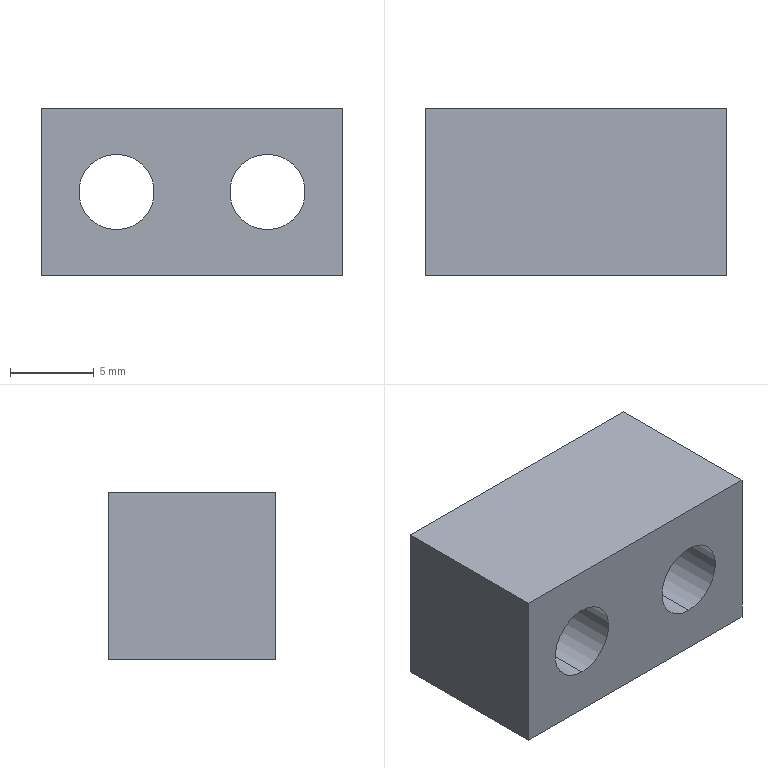Part | STEP file | limit block | 1 solid | 16 faces | box 18 x 10 x 10 mm | volume 1180 mm3 | cylinder 8 | plane 8 | commonest cylinder face diameters 4.5 x4 8 x4
STEP:
#1=CARTESIAN_POINT('',(0.,0.,0.));
#2=DIRECTION('',(0.,0.,1.));
#3=DIRECTION('',(1.,0.,0.));
#4=AXIS2_PLACEMENT_3D('',#1,#2,#3);
#5=CARTESIAN_POINT('',(-4.5,5.6,4.));
#6=VERTEX_POINT('',#5);
#7=CARTESIAN_POINT('',(-4.5,10.,4.));
#8=VERTEX_POINT('',#7);
#9=CARTESIAN_POINT('',(-4.5,10.,4.));
#10=DIRECTION('',(0.,1.,0.));
#11=VECTOR('',#10,1.);
#12=LINE('',#9,#11);
#13=CARTESIAN_POINT('',(-4.5,10.,0.));
#14=DIRECTION('',(0.,1.,0.));
#15=DIRECTION('',(0.,0.,1.));
#16=AXIS2_PLACEMENT_3D('',#13,#14,#15);
#17=CYLINDRICAL_SURFACE('',#16,4.);
#18=CARTESIAN_POINT('',(6.283,0.));
#19=DIRECTION('',(0.,1.));
#20=VECTOR('',#19,1.);
#21=LINE('',#18,#20);
#22=(GEOMETRIC_REPRESENTATION_CONTEXT(2)PARAMETRIC_REPRESENTATION_CONTEXT()REPRESENTATION_CONTEXT('',''));
#23=DEFINITIONAL_REPRESENTATION('',(#21),#22);
#24=PCURVE('',#17,#23);
#25=CARTESIAN_POINT('',(-4.5,10.,0.));
#26=DIRECTION('',(0.,1.,0.));
#27=DIRECTION('',(0.,0.,1.));
#28=AXIS2_PLACEMENT_3D('',#25,#26,#27);
#29=CYLINDRICAL_SURFACE('',#28,4.);
#30=CARTESIAN_POINT('',(0.,0.));
#31=DIRECTION('',(0.,1.));
#32=VECTOR('',#31,1.);
#33=LINE('',#30,#32);
#34=(GEOMETRIC_REPRESENTATION_CONTEXT(2)PARAMETRIC_REPRESENTATION_CONTEXT()REPRESENTATION_CONTEXT('',''));
#35=DEFINITIONAL_REPRESENTATION('',(#33),#34);
#36=PCURVE('',#29,#35);
#37=SURFACE_CURVE('',#12,(#24,#36),.PCURVE_S1.);
#38=EDGE_CURVE('',#6,#8,#37,.T.);
#39=ORIENTED_EDGE('',*,*,#38,.T.);
#40=CARTESIAN_POINT('',(-4.5,10.,-4.));
#41=VERTEX_POINT('',#40);
#42=CARTESIAN_POINT('',(-4.5,10.,0.));
#43=DIRECTION('',(0.,1.,0.));
#44=DIRECTION('',(0.,0.,1.));
#45=AXIS2_PLACEMENT_3D('',#42,#43,#44);
#46=CIRCLE('',#45,4.);
#47=CARTESIAN_POINT('',(0.,0.));
#48=DIRECTION('',(1.,0.));
#49=VECTOR('',#48,1.);
#50=LINE('',#47,#49);
#51=(GEOMETRIC_REPRESENTATION_CONTEXT(2)PARAMETRIC_REPRESENTATION_CONTEXT()REPRESENTATION_CONTEXT('',''));
#52=DEFINITIONAL_REPRESENTATION('',(#50),#51);
#53=PCURVE('',#17,#52);
#54=CARTESIAN_POINT('',(0.,10.,0.));
#55=DIRECTION('',(0.,1.,0.));
#56=DIRECTION('',(0.,0.,1.));
#57=AXIS2_PLACEMENT_3D('',#54,#55,#56);
#58=PLANE('',#57);
#59=CARTESIAN_POINT('',(0.,-4.5));
#60=DIRECTION('',(1.,0.));
#61=AXIS2_PLACEMENT_2D('',#59,#60);
#62=CIRCLE('',#61,4.);
#63=(GEOMETRIC_REPRESENTATION_CONTEXT(2)PARAMETRIC_REPRESENTATION_CONTEXT()REPRESENTATION_CONTEXT('',''));
#64=DEFINITIONAL_REPRESENTATION('',(#62),#63);
#65=PCURVE('',#58,#64);
#66=SURFACE_CURVE('',#46,(#53,#65),.PCURVE_S1.);
#67=EDGE_CURVE('',#41,#8,#66,.T.);
#68=ORIENTED_EDGE('',*,*,#67,.F.);
#69=CARTESIAN_POINT('',(-4.5,5.6,-4.));
#70=VERTEX_POINT('',#69);
#71=CARTESIAN_POINT('',(-4.5,10.,-4.));
#72=DIRECTION('',(0.,1.,0.));
#73=VECTOR('',#72,1.);
#74=LINE('',#71,#73);
#75=CARTESIAN_POINT('',(3.142,0.));
#76=DIRECTION('',(0.,1.));
#77=VECTOR('',#76,1.);
#78=LINE('',#75,#77);
#79=(GEOMETRIC_REPRESENTATION_CONTEXT(2)PARAMETRIC_REPRESENTATION_CONTEXT()REPRESENTATION_CONTEXT('',''));
#80=DEFINITIONAL_REPRESENTATION('',(#78),#79);
#81=PCURVE('',#17,#80);
#82=CARTESIAN_POINT('',(3.142,0.));
#83=DIRECTION('',(0.,1.));
#84=VECTOR('',#83,1.);
#85=LINE('',#82,#84);
#86=(GEOMETRIC_REPRESENTATION_CONTEXT(2)PARAMETRIC_REPRESENTATION_CONTEXT()REPRESENTATION_CONTEXT('',''));
#87=DEFINITIONAL_REPRESENTATION('',(#85),#86);
#88=PCURVE('',#29,#87);
#89=SURFACE_CURVE('',#74,(#81,#88),.PCURVE_S1.);
#90=EDGE_CURVE('',#70,#41,#89,.T.);
#91=ORIENTED_EDGE('',*,*,#90,.F.);
#92=CARTESIAN_POINT('',(-4.5,5.6,0.));
#93=DIRECTION('',(0.,1.,0.));
#94=DIRECTION('',(0.,0.,1.));
#95=AXIS2_PLACEMENT_3D('',#92,#93,#94);
#96=CIRCLE('',#95,4.);
#97=CARTESIAN_POINT('',(0.,-4.4));
#98=DIRECTION('',(1.,0.));
#99=VECTOR('',#98,1.);
#100=LINE('',#97,#99);
#101=(GEOMETRIC_REPRESENTATION_CONTEXT(2)PARAMETRIC_REPRESENTATION_CONTEXT()REPRESENTATION_CONTEXT('',''));
#102=DEFINITIONAL_REPRESENTATION('',(#100),#101);
#103=PCURVE('',#17,#102);
#104=CARTESIAN_POINT('',(-2.25,5.6,0.));
#105=DIRECTION('',(0.,-1.,0.));
#106=DIRECTION('',(0.,0.,-1.));
#107=AXIS2_PLACEMENT_3D('',#104,#105,#106);
#108=PLANE('',#107);
#109=CARTESIAN_POINT('',(-4.,-2.25));
#110=CARTESIAN_POINT('',(-4.,4.678));
#111=CARTESIAN_POINT('',(2.,1.214));
#112=CARTESIAN_POINT('',(8.,-2.25));
#113=CARTESIAN_POINT('',(2.,-5.714));
#114=CARTESIAN_POINT('',(-4.,-9.178));
#115=CARTESIAN_POINT('',(-4.,-2.25));
#116=(BOUNDED_CURVE()B_SPLINE_CURVE(2,(#109,#110,#111,#112,#113,#114,#115),.UNSPECIFIED.,.T.,.F.)B_SPLINE_CURVE_WITH_KNOTS((1,2,2,2,2,1),(-2.094,0.,2.094,4.189,6.283,8.378),.UNSPECIFIED.)CURVE()GEOMETRIC_REPRESENTATION_ITEM()RATIONAL_B_SPLINE_CURVE((1.,0.5,1.,0.5,1.,0.5,1.))REPRESENTATION_ITEM(''));
#117=(GEOMETRIC_REPRESENTATION_CONTEXT(2)PARAMETRIC_REPRESENTATION_CONTEXT()REPRESENTATION_CONTEXT('',''));
#118=DEFINITIONAL_REPRESENTATION('',(#116),#117);
#119=PCURVE('',#108,#118);
#120=SURFACE_CURVE('',#96,(#103,#119),.PCURVE_S1.);
#121=EDGE_CURVE('',#70,#6,#120,.T.);
#122=ORIENTED_EDGE('',*,*,#121,.T.);
#123=EDGE_LOOP('',(#39,#68,#91,#122));
#124=FACE_BOUND('',#123,.F.);
#125=ADVANCED_FACE('',(#124),#17,.F.);
#126=CARTESIAN_POINT('',(-4.5,0.,2.25));
#127=VERTEX_POINT('',#126);
#128=CARTESIAN_POINT('',(-4.5,5.6,2.25));
#129=VERTEX_POINT('',#128);
#130=CARTESIAN_POINT('',(-4.5,10.,2.25));
#131=DIRECTION('',(0.,1.,0.));
#132=VECTOR('',#131,1.);
#133=LINE('',#130,#132);
#134=CARTESIAN_POINT('',(-4.5,10.,0.));
#135=DIRECTION('',(0.,1.,0.));
#136=DIRECTION('',(0.,0.,1.));
#137=AXIS2_PLACEMENT_3D('',#134,#135,#136);
#138=CYLINDRICAL_SURFACE('',#137,2.25);
#139=CARTESIAN_POINT('',(6.283,0.));
#140=DIRECTION('',(0.,1.));
#141=VECTOR('',#140,1.);
#142=LINE('',#139,#141);
#143=(GEOMETRIC_REPRESENTATION_CONTEXT(2)PARAMETRIC_REPRESENTATION_CONTEXT()REPRESENTATION_CONTEXT('',''));
#144=DEFINITIONAL_REPRESENTATION('',(#142),#143);
#145=PCURVE('',#138,#144);
#146=CARTESIAN_POINT('',(-4.5,10.,0.));
#147=DIRECTION('',(0.,1.,0.));
#148=DIRECTION('',(0.,0.,1.));
#149=AXIS2_PLACEMENT_3D('',#146,#147,#148);
#150=CYLINDRICAL_SURFACE('',#149,2.25);
#151=CARTESIAN_POINT('',(0.,0.));
#152=DIRECTION('',(0.,1.));
#153=VECTOR('',#152,1.);
#154=LINE('',#151,#153);
#155=(GEOMETRIC_REPRESENTATION_CONTEXT(2)PARAMETRIC_REPRESENTATION_CONTEXT()REPRESENTATION_CONTEXT('',''));
#156=DEFINITIONAL_REPRESENTATION('',(#154),#155);
#157=PCURVE('',#150,#156);
#158=SURFACE_CURVE('',#133,(#145,#157),.PCURVE_S1.);
#159=EDGE_CURVE('',#127,#129,#158,.T.);
#160=ORIENTED_EDGE('',*,*,#159,.T.);
#161=CARTESIAN_POINT('',(-4.5,5.6,-2.25));
#162=VERTEX_POINT('',#161);
#163=CARTESIAN_POINT('',(-4.5,5.6,0.));
#164=DIRECTION('',(0.,1.,0.));
#165=DIRECTION('',(0.,0.,1.));
#166=AXIS2_PLACEMENT_3D('',#163,#164,#165);
#167=CIRCLE('',#166,2.25);
#168=CARTESIAN_POINT('',(0.,-4.4));
#169=DIRECTION('',(1.,0.));
#170=VECTOR('',#169,1.);
#171=LINE('',#168,#170);
#172=(GEOMETRIC_REPRESENTATION_CONTEXT(2)PARAMETRIC_REPRESENTATION_CONTEXT()REPRESENTATION_CONTEXT('',''));
#173=DEFINITIONAL_REPRESENTATION('',(#171),#172);
#174=PCURVE('',#138,#173);
#175=CARTESIAN_POINT('',(-2.25,-2.25));
#176=CARTESIAN_POINT('',(-2.25,1.647));
#177=CARTESIAN_POINT('',(1.125,-0.3014));
#178=CARTESIAN_POINT('',(4.5,-2.25));
#179=CARTESIAN_POINT('',(1.125,-4.199));
#180=CARTESIAN_POINT('',(-2.25,-6.147));
#181=CARTESIAN_POINT('',(-2.25,-2.25));
#182=(BOUNDED_CURVE()B_SPLINE_CURVE(2,(#175,#176,#177,#178,#179,#180,#181),.UNSPECIFIED.,.T.,.F.)B_SPLINE_CURVE_WITH_KNOTS((1,2,2,2,2,1),(-2.094,0.,2.094,4.189,6.283,8.378),.UNSPECIFIED.)CURVE()GEOMETRIC_REPRESENTATION_ITEM()RATIONAL_B_SPLINE_CURVE((1.,0.5,1.,0.5,1.,0.5,1.))REPRESENTATION_ITEM(''));
#183=(GEOMETRIC_REPRESENTATION_CONTEXT(2)PARAMETRIC_REPRESENTATION_CONTEXT()REPRESENTATION_CONTEXT('',''));
#184=DEFINITIONAL_REPRESENTATION('',(#182),#183);
#185=PCURVE('',#108,#184);
#186=SURFACE_CURVE('',#167,(#174,#185),.PCURVE_S1.);
#187=EDGE_CURVE('',#162,#129,#186,.T.);
#188=ORIENTED_EDGE('',*,*,#187,.F.);
#189=CARTESIAN_POINT('',(-4.5,0.,-2.25));
#190=VERTEX_POINT('',#189);
#191=CARTESIAN_POINT('',(-4.5,10.,-2.25));
#192=DIRECTION('',(0.,1.,0.));
#193=VECTOR('',#192,1.);
#194=LINE('',#191,#193);
#195=CARTESIAN_POINT('',(3.142,0.));
#196=DIRECTION('',(0.,1.));
#197=VECTOR('',#196,1.);
#198=LINE('',#195,#197);
#199=(GEOMETRIC_REPRESENTATION_CONTEXT(2)PARAMETRIC_REPRESENTATION_CONTEXT()REPRESENTATION_CONTEXT('',''));
#200=DEFINITIONAL_REPRESENTATION('',(#198),#199);
#201=PCURVE('',#138,#200);
#202=CARTESIAN_POINT('',(3.142,0.));
#203=DIRECTION('',(0.,1.));
#204=VECTOR('',#203,1.);
#205=LINE('',#202,#204);
#206=(GEOMETRIC_REPRESENTATION_CONTEXT(2)PARAMETRIC_REPRESENTATION_CONTEXT()REPRESENTATION_CONTEXT('',''));
#207=DEFINITIONAL_REPRESENTATION('',(#205),#206);
#208=PCURVE('',#150,#207);
#209=SURFACE_CURVE('',#194,(#201,#208),.PCURVE_S1.);
#210=EDGE_CURVE('',#190,#162,#209,.T.);
#211=ORIENTED_EDGE('',*,*,#210,.F.);
#212=CARTESIAN_POINT('',(-4.5,0.,0.));
#213=DIRECTION('',(0.,1.,0.));
#214=DIRECTION('',(0.,0.,1.));
#215=AXIS2_PLACEMENT_3D('',#212,#213,#214);
#216=CIRCLE('',#215,2.25);
#217=CARTESIAN_POINT('',(0.,-10.));
#218=DIRECTION('',(1.,0.));
#219=VECTOR('',#218,1.);
#220=LINE('',#217,#219);
#221=(GEOMETRIC_REPRESENTATION_CONTEXT(2)PARAMETRIC_REPRESENTATION_CONTEXT()REPRESENTATION_CONTEXT('',''));
#222=DEFINITIONAL_REPRESENTATION('',(#220),#221);
#223=PCURVE('',#138,#222);
#224=CARTESIAN_POINT('',(0.,0.,0.));
#225=DIRECTION('',(0.,1.,0.));
#226=DIRECTION('',(0.,0.,1.));
#227=AXIS2_PLACEMENT_3D('',#224,#225,#226);
#228=PLANE('',#227);
#229=CARTESIAN_POINT('',(0.,-4.5));
#230=DIRECTION('',(1.,0.));
#231=AXIS2_PLACEMENT_2D('',#229,#230);
#232=CIRCLE('',#231,2.25);
#233=(GEOMETRIC_REPRESENTATION_CONTEXT(2)PARAMETRIC_REPRESENTATION_CONTEXT()REPRESENTATION_CONTEXT('',''));
#234=DEFINITIONAL_REPRESENTATION('',(#232),#233);
#235=PCURVE('',#228,#234);
#236=SURFACE_CURVE('',#216,(#223,#235),.PCURVE_S1.);
#237=EDGE_CURVE('',#190,#127,#236,.T.);
#238=ORIENTED_EDGE('',*,*,#237,.T.);
#239=EDGE_LOOP('',(#160,#188,#211,#238));
#240=FACE_BOUND('',#239,.F.);
#241=ADVANCED_FACE('',(#240),#138,.F.);
#242=CARTESIAN_POINT('',(4.5,5.6,4.));
#243=VERTEX_POINT('',#242);
#244=CARTESIAN_POINT('',(4.5,10.,4.));
#245=VERTEX_POINT('',#244);
#246=CARTESIAN_POINT('',(4.5,10.,4.));
#247=DIRECTION('',(0.,1.,0.));
#248=VECTOR('',#247,1.);
#249=LINE('',#246,#248);
#250=CARTESIAN_POINT('',(4.5,10.,0.));
#251=DIRECTION('',(0.,1.,0.));
#252=DIRECTION('',(0.,0.,1.));
#253=AXIS2_PLACEMENT_3D('',#250,#251,#252);
#254=CYLINDRICAL_SURFACE('',#253,4.);
#255=CARTESIAN_POINT('',(6.283,0.));
#256=DIRECTION('',(0.,1.));
#257=VECTOR('',#256,1.);
#258=LINE('',#255,#257);
#259=(GEOMETRIC_REPRESENTATION_CONTEXT(2)PARAMETRIC_REPRESENTATION_CONTEXT()REPRESENTATION_CONTEXT('',''));
#260=DEFINITIONAL_REPRESENTATION('',(#258),#259);
#261=PCURVE('',#254,#260);
#262=CARTESIAN_POINT('',(4.5,10.,0.));
#263=DIRECTION('',(0.,1.,0.));
#264=DIRECTION('',(0.,0.,1.));
#265=AXIS2_PLACEMENT_3D('',#262,#263,#264);
#266=CYLINDRICAL_SURFACE('',#265,4.);
#267=CARTESIAN_POINT('',(0.,0.));
#268=DIRECTION('',(0.,1.));
#269=VECTOR('',#268,1.);
#270=LINE('',#267,#269);
#271=(GEOMETRIC_REPRESENTATION_CONTEXT(2)PARAMETRIC_REPRESENTATION_CONTEXT()REPRESENTATION_CONTEXT('',''));
#272=DEFINITIONAL_REPRESENTATION('',(#270),#271);
#273=PCURVE('',#266,#272);
#274=SURFACE_CURVE('',#249,(#261,#273),.PCURVE_S1.);
#275=EDGE_CURVE('',#243,#245,#274,.T.);
#276=ORIENTED_EDGE('',*,*,#275,.T.);
#277=CARTESIAN_POINT('',(4.5,10.,-4.));
#278=VERTEX_POINT('',#277);
#279=CARTESIAN_POINT('',(4.5,10.,0.));
#280=DIRECTION('',(0.,1.,0.));
#281=DIRECTION('',(0.,0.,1.));
#282=AXIS2_PLACEMENT_3D('',#279,#280,#281);
#283=CIRCLE('',#282,4.);
#284=CARTESIAN_POINT('',(0.,0.));
#285=DIRECTION('',(1.,0.));
#286=VECTOR('',#285,1.);
#287=LINE('',#284,#286);
#288=(GEOMETRIC_REPRESENTATION_CONTEXT(2)PARAMETRIC_REPRESENTATION_CONTEXT()REPRESENTATION_CONTEXT('',''));
#289=DEFINITIONAL_REPRESENTATION('',(#287),#288);
#290=PCURVE('',#254,#289);
#291=CARTESIAN_POINT('',(0.,4.5));
#292=DIRECTION('',(1.,0.));
#293=AXIS2_PLACEMENT_2D('',#291,#292);
#294=CIRCLE('',#293,4.);
#295=(GEOMETRIC_REPRESENTATION_CONTEXT(2)PARAMETRIC_REPRESENTATION_CONTEXT()REPRESENTATION_CONTEXT('',''));
#296=DEFINITIONAL_REPRESENTATION('',(#294),#295);
#297=PCURVE('',#58,#296);
#298=SURFACE_CURVE('',#283,(#290,#297),.PCURVE_S1.);
#299=EDGE_CURVE('',#278,#245,#298,.T.);
#300=ORIENTED_EDGE('',*,*,#299,.F.);
#301=CARTESIAN_POINT('',(4.5,5.6,-4.));
#302=VERTEX_POINT('',#301);
#303=CARTESIAN_POINT('',(4.5,10.,-4.));
#304=DIRECTION('',(0.,1.,0.));
#305=VECTOR('',#304,1.);
#306=LINE('',#303,#305);
#307=CARTESIAN_POINT('',(3.142,0.));
#308=DIRECTION('',(0.,1.));
#309=VECTOR('',#308,1.);
#310=LINE('',#307,#309);
#311=(GEOMETRIC_REPRESENTATION_CONTEXT(2)PARAMETRIC_REPRESENTATION_CONTEXT()REPRESENTATION_CONTEXT('',''));
#312=DEFINITIONAL_REPRESENTATION('',(#310),#311);
#313=PCURVE('',#254,#312);
#314=CARTESIAN_POINT('',(3.142,0.));
#315=DIRECTION('',(0.,1.));
#316=VECTOR('',#315,1.);
#317=LINE('',#314,#316);
#318=(GEOMETRIC_REPRESENTATION_CONTEXT(2)PARAMETRIC_REPRESENTATION_CONTEXT()REPRESENTATION_CONTEXT('',''));
#319=DEFINITIONAL_REPRESENTATION('',(#317),#318);
#320=PCURVE('',#266,#319);
#321=SURFACE_CURVE('',#306,(#313,#320),.PCURVE_S1.);
#322=EDGE_CURVE('',#302,#278,#321,.T.);
#323=ORIENTED_EDGE('',*,*,#322,.F.);
#324=CARTESIAN_POINT('',(4.5,5.6,0.));
#325=DIRECTION('',(0.,1.,0.));
#326=DIRECTION('',(0.,0.,1.));
#327=AXIS2_PLACEMENT_3D('',#324,#325,#326);
#328=CIRCLE('',#327,4.);
#329=CARTESIAN_POINT('',(0.,-4.4));
#330=DIRECTION('',(1.,0.));
#331=VECTOR('',#330,1.);
#332=LINE('',#329,#331);
#333=(GEOMETRIC_REPRESENTATION_CONTEXT(2)PARAMETRIC_REPRESENTATION_CONTEXT()REPRESENTATION_CONTEXT('',''));
#334=DEFINITIONAL_REPRESENTATION('',(#332),#333);
#335=PCURVE('',#254,#334);
#336=CARTESIAN_POINT('',(6.75,5.6,0.));
#337=DIRECTION('',(0.,-1.,0.));
#338=DIRECTION('',(0.,0.,-1.));
#339=AXIS2_PLACEMENT_3D('',#336,#337,#338);
#340=PLANE('',#339);
#341=CARTESIAN_POINT('',(-4.,-2.25));
#342=CARTESIAN_POINT('',(-4.,4.678));
#343=CARTESIAN_POINT('',(2.,1.214));
#344=CARTESIAN_POINT('',(8.,-2.25));
#345=CARTESIAN_POINT('',(2.,-5.714));
#346=CARTESIAN_POINT('',(-4.,-9.178));
#347=CARTESIAN_POINT('',(-4.,-2.25));
#348=(BOUNDED_CURVE()B_SPLINE_CURVE(2,(#341,#342,#343,#344,#345,#346,#347),.UNSPECIFIED.,.T.,.F.)B_SPLINE_CURVE_WITH_KNOTS((1,2,2,2,2,1),(-2.094,0.,2.094,4.189,6.283,8.378),.UNSPECIFIED.)CURVE()GEOMETRIC_REPRESENTATION_ITEM()RATIONAL_B_SPLINE_CURVE((1.,0.5,1.,0.5,1.,0.5,1.))REPRESENTATION_ITEM(''));
#349=(GEOMETRIC_REPRESENTATION_CONTEXT(2)PARAMETRIC_REPRESENTATION_CONTEXT()REPRESENTATION_CONTEXT('',''));
#350=DEFINITIONAL_REPRESENTATION('',(#348),#349);
#351=PCURVE('',#340,#350);
#352=SURFACE_CURVE('',#328,(#335,#351),.PCURVE_S1.);
#353=EDGE_CURVE('',#302,#243,#352,.T.);
#354=ORIENTED_EDGE('',*,*,#353,.T.);
#355=EDGE_LOOP('',(#276,#300,#323,#354));
#356=FACE_BOUND('',#355,.F.);
#357=ADVANCED_FACE('',(#356),#254,.F.);
#358=CARTESIAN_POINT('',(4.5,0.,2.25));
#359=VERTEX_POINT('',#358);
#360=CARTESIAN_POINT('',(4.5,5.6,2.25));
#361=VERTEX_POINT('',#360);
#362=CARTESIAN_POINT('',(4.5,10.,2.25));
#363=DIRECTION('',(0.,1.,0.));
#364=VECTOR('',#363,1.);
#365=LINE('',#362,#364);
#366=CARTESIAN_POINT('',(4.5,10.,0.));
#367=DIRECTION('',(0.,1.,0.));
#368=DIRECTION('',(0.,0.,1.));
#369=AXIS2_PLACEMENT_3D('',#366,#367,#368);
#370=CYLINDRICAL_SURFACE('',#369,2.25);
#371=CARTESIAN_POINT('',(6.283,0.));
#372=DIRECTION('',(0.,1.));
#373=VECTOR('',#372,1.);
#374=LINE('',#371,#373);
#375=(GEOMETRIC_REPRESENTATION_CONTEXT(2)PARAMETRIC_REPRESENTATION_CONTEXT()REPRESENTATION_CONTEXT('',''));
#376=DEFINITIONAL_REPRESENTATION('',(#374),#375);
#377=PCURVE('',#370,#376);
#378=CARTESIAN_POINT('',(4.5,10.,0.));
#379=DIRECTION('',(0.,1.,0.));
#380=DIRECTION('',(0.,0.,1.));
#381=AXIS2_PLACEMENT_3D('',#378,#379,#380);
#382=CYLINDRICAL_SURFACE('',#381,2.25);
#383=CARTESIAN_POINT('',(0.,0.));
#384=DIRECTION('',(0.,1.));
#385=VECTOR('',#384,1.);
#386=LINE('',#383,#385);
#387=(GEOMETRIC_REPRESENTATION_CONTEXT(2)PARAMETRIC_REPRESENTATION_CONTEXT()REPRESENTATION_CONTEXT('',''));
#388=DEFINITIONAL_REPRESENTATION('',(#386),#387);
#389=PCURVE('',#382,#388);
#390=SURFACE_CURVE('',#365,(#377,#389),.PCURVE_S1.);
#391=EDGE_CURVE('',#359,#361,#390,.T.);
#392=ORIENTED_EDGE('',*,*,#391,.T.);
#393=CARTESIAN_POINT('',(4.5,5.6,-2.25));
#394=VERTEX_POINT('',#393);
#395=CARTESIAN_POINT('',(4.5,5.6,0.));
#396=DIRECTION('',(0.,1.,0.));
#397=DIRECTION('',(0.,0.,1.));
#398=AXIS2_PLACEMENT_3D('',#395,#396,#397);
#399=CIRCLE('',#398,2.25);
#400=CARTESIAN_POINT('',(0.,-4.4));
#401=DIRECTION('',(1.,0.));
#402=VECTOR('',#401,1.);
#403=LINE('',#400,#402);
#404=(GEOMETRIC_REPRESENTATION_CONTEXT(2)PARAMETRIC_REPRESENTATION_CONTEXT()REPRESENTATION_CONTEXT('',''));
#405=DEFINITIONAL_REPRESENTATION('',(#403),#404);
#406=PCURVE('',#370,#405);
#407=CARTESIAN_POINT('',(-2.25,-2.25));
#408=CARTESIAN_POINT('',(-2.25,1.647));
#409=CARTESIAN_POINT('',(1.125,-0.3014));
#410=CARTESIAN_POINT('',(4.5,-2.25));
#411=CARTESIAN_POINT('',(1.125,-4.199));
#412=CARTESIAN_POINT('',(-2.25,-6.147));
#413=CARTESIAN_POINT('',(-2.25,-2.25));
#414=(BOUNDED_CURVE()B_SPLINE_CURVE(2,(#407,#408,#409,#410,#411,#412,#413),.UNSPECIFIED.,.T.,.F.)B_SPLINE_CURVE_WITH_KNOTS((1,2,2,2,2,1),(-2.094,0.,2.094,4.189,6.283,8.378),.UNSPECIFIED.)CURVE()GEOMETRIC_REPRESENTATION_ITEM()RATIONAL_B_SPLINE_CURVE((1.,0.5,1.,0.5,1.,0.5,1.))REPRESENTATION_ITEM(''));
#415=(GEOMETRIC_REPRESENTATION_CONTEXT(2)PARAMETRIC_REPRESENTATION_CONTEXT()REPRESENTATION_CONTEXT('',''));
#416=DEFINITIONAL_REPRESENTATION('',(#414),#415);
#417=PCURVE('',#340,#416);
#418=SURFACE_CURVE('',#399,(#406,#417),.PCURVE_S1.);
#419=EDGE_CURVE('',#394,#361,#418,.T.);
#420=ORIENTED_EDGE('',*,*,#419,.F.);
#421=CARTESIAN_POINT('',(4.5,0.,-2.25));
#422=VERTEX_POINT('',#421);
#423=CARTESIAN_POINT('',(4.5,10.,-2.25));
#424=DIRECTION('',(0.,1.,0.));
#425=VECTOR('',#424,1.);
#426=LINE('',#423,#425);
#427=CARTESIAN_POINT('',(3.142,0.));
#428=DIRECTION('',(0.,1.));
#429=VECTOR('',#428,1.);
#430=LINE('',#427,#429);
#431=(GEOMETRIC_REPRESENTATION_CONTEXT(2)PARAMETRIC_REPRESENTATION_CONTEXT()REPRESENTATION_CONTEXT('',''));
#432=DEFINITIONAL_REPRESENTATION('',(#430),#431);
#433=PCURVE('',#370,#432);
#434=CARTESIAN_POINT('',(3.142,0.));
#435=DIRECTION('',(0.,1.));
#436=VECTOR('',#435,1.);
#437=LINE('',#434,#436);
#438=(GEOMETRIC_REPRESENTATION_CONTEXT(2)PARAMETRIC_REPRESENTATION_CONTEXT()REPRESENTATION_CONTEXT('',''));
#439=DEFINITIONAL_REPRESENTATION('',(#437),#438);
#440=PCURVE('',#382,#439);
#441=SURFACE_CURVE('',#426,(#433,#440),.PCURVE_S1.);
#442=EDGE_CURVE('',#422,#394,#441,.T.);
#443=ORIENTED_EDGE('',*,*,#442,.F.);
#444=CARTESIAN_POINT('',(4.5,0.,0.));
#445=DIRECTION('',(0.,1.,0.));
#446=DIRECTION('',(0.,0.,1.));
#447=AXIS2_PLACEMENT_3D('',#444,#445,#446);
#448=CIRCLE('',#447,2.25);
#449=CARTESIAN_POINT('',(0.,-10.));
#450=DIRECTION('',(1.,0.));
#451=VECTOR('',#450,1.);
#452=LINE('',#449,#451);
#453=(GEOMETRIC_REPRESENTATION_CONTEXT(2)PARAMETRIC_REPRESENTATION_CONTEXT()REPRESENTATION_CONTEXT('',''));
#454=DEFINITIONAL_REPRESENTATION('',(#452),#453);
#455=PCURVE('',#370,#454);
#456=CARTESIAN_POINT('',(0.,4.5));
#457=DIRECTION('',(1.,0.));
#458=AXIS2_PLACEMENT_2D('',#456,#457);
#459=CIRCLE('',#458,2.25);
#460=(GEOMETRIC_REPRESENTATION_CONTEXT(2)PARAMETRIC_REPRESENTATION_CONTEXT()REPRESENTATION_CONTEXT('',''));
#461=DEFINITIONAL_REPRESENTATION('',(#459),#460);
#462=PCURVE('',#228,#461);
#463=SURFACE_CURVE('',#448,(#455,#462),.PCURVE_S1.);
#464=EDGE_CURVE('',#422,#359,#463,.T.);
#465=ORIENTED_EDGE('',*,*,#464,.T.);
#466=EDGE_LOOP('',(#392,#420,#443,#465));
#467=FACE_BOUND('',#466,.F.);
#468=ADVANCED_FACE('',(#467),#370,.F.);
#469=CARTESIAN_POINT('',(9.,0.,5.));
#470=VERTEX_POINT('',#469);
#471=CARTESIAN_POINT('',(9.,0.,-5.));
#472=VERTEX_POINT('',#471);
#473=CARTESIAN_POINT('',(9.,0.,-5.));
#474=DIRECTION('',(0.,0.,-1.));
#475=VECTOR('',#474,1.);
#476=LINE('',#473,#475);
#477=CARTESIAN_POINT('',(9.,10.,-5.));
#478=DIRECTION('',(-1.,0.,0.));
#479=DIRECTION('',(0.,0.,1.));
#480=AXIS2_PLACEMENT_3D('',#477,#478,#479);
#481=PLANE('',#480);
#482=CARTESIAN_POINT('',(0.,-10.));
#483=DIRECTION('',(-1.,0.));
#484=VECTOR('',#483,1.);
#485=LINE('',#482,#484);
#486=(GEOMETRIC_REPRESENTATION_CONTEXT(2)PARAMETRIC_REPRESENTATION_CONTEXT()REPRESENTATION_CONTEXT('',''));
#487=DEFINITIONAL_REPRESENTATION('',(#485),#486);
#488=PCURVE('',#481,#487);
#489=CARTESIAN_POINT('',(-5.,9.));
#490=DIRECTION('',(-1.,0.));
#491=VECTOR('',#490,1.);
#492=LINE('',#489,#491);
#493=(GEOMETRIC_REPRESENTATION_CONTEXT(2)PARAMETRIC_REPRESENTATION_CONTEXT()REPRESENTATION_CONTEXT('',''));
#494=DEFINITIONAL_REPRESENTATION('',(#492),#493);
#495=PCURVE('',#228,#494);
#496=SURFACE_CURVE('',#476,(#488,#495),.PCURVE_S1.);
#497=EDGE_CURVE('',#470,#472,#496,.T.);
#498=ORIENTED_EDGE('',*,*,#497,.T.);
#499=CARTESIAN_POINT('',(9.,10.,-5.));
#500=VERTEX_POINT('',#499);
#501=CARTESIAN_POINT('',(9.,10.,-5.));
#502=DIRECTION('',(0.,-1.,0.));
#503=VECTOR('',#502,1.);
#504=LINE('',#501,#503);
#505=CARTESIAN_POINT('',(0.,0.));
#506=DIRECTION('',(0.,-1.));
#507=VECTOR('',#506,1.);
#508=LINE('',#505,#507);
#509=(GEOMETRIC_REPRESENTATION_CONTEXT(2)PARAMETRIC_REPRESENTATION_CONTEXT()REPRESENTATION_CONTEXT('',''));
#510=DEFINITIONAL_REPRESENTATION('',(#508),#509);
#511=PCURVE('',#481,#510);
#512=CARTESIAN_POINT('',(-9.,10.,-5.));
#513=DIRECTION('',(0.,0.,1.));
#514=DIRECTION('',(1.,0.,0.));
#515=AXIS2_PLACEMENT_3D('',#512,#513,#514);
#516=PLANE('',#515);
#517=CARTESIAN_POINT('',(18.,0.));
#518=DIRECTION('',(0.,-1.));
#519=VECTOR('',#518,1.);
#520=LINE('',#517,#519);
#521=(GEOMETRIC_REPRESENTATION_CONTEXT(2)PARAMETRIC_REPRESENTATION_CONTEXT()REPRESENTATION_CONTEXT('',''));
#522=DEFINITIONAL_REPRESENTATION('',(#520),#521);
#523=PCURVE('',#516,#522);
#524=SURFACE_CURVE('',#504,(#511,#523),.PCURVE_S1.);
#525=EDGE_CURVE('',#500,#472,#524,.T.);
#526=ORIENTED_EDGE('',*,*,#525,.F.);
#527=CARTESIAN_POINT('',(9.,10.,5.));
#528=VERTEX_POINT('',#527);
#529=CARTESIAN_POINT('',(9.,10.,-5.));
#530=DIRECTION('',(0.,0.,-1.));
#531=VECTOR('',#530,1.);
#532=LINE('',#529,#531);
#533=CARTESIAN_POINT('',(0.,0.));
#534=DIRECTION('',(-1.,0.));
#535=VECTOR('',#534,1.);
#536=LINE('',#533,#535);
#537=(GEOMETRIC_REPRESENTATION_CONTEXT(2)PARAMETRIC_REPRESENTATION_CONTEXT()REPRESENTATION_CONTEXT('',''));
#538=DEFINITIONAL_REPRESENTATION('',(#536),#537);
#539=PCURVE('',#481,#538);
#540=CARTESIAN_POINT('',(-5.,9.));
#541=DIRECTION('',(-1.,0.));
#542=VECTOR('',#541,1.);
#543=LINE('',#540,#542);
#544=(GEOMETRIC_REPRESENTATION_CONTEXT(2)PARAMETRIC_REPRESENTATION_CONTEXT()REPRESENTATION_CONTEXT('',''));
#545=DEFINITIONAL_REPRESENTATION('',(#543),#544);
#546=PCURVE('',#58,#545);
#547=SURFACE_CURVE('',#532,(#539,#546),.PCURVE_S1.);
#548=EDGE_CURVE('',#528,#500,#547,.T.);
#549=ORIENTED_EDGE('',*,*,#548,.F.);
#550=CARTESIAN_POINT('',(9.,10.,5.));
#551=DIRECTION('',(0.,-1.,0.));
#552=VECTOR('',#551,1.);
#553=LINE('',#550,#552);
#554=CARTESIAN_POINT('',(10.,0.));
#555=DIRECTION('',(0.,-1.));
#556=VECTOR('',#555,1.);
#557=LINE('',#554,#556);
#558=(GEOMETRIC_REPRESENTATION_CONTEXT(2)PARAMETRIC_REPRESENTATION_CONTEXT()REPRESENTATION_CONTEXT('',''));
#559=DEFINITIONAL_REPRESENTATION('',(#557),#558);
#560=PCURVE('',#481,#559);
#561=CARTESIAN_POINT('',(-9.,10.,5.));
#562=DIRECTION('',(0.,0.,-1.));
#563=DIRECTION('',(-1.,0.,0.));
#564=AXIS2_PLACEMENT_3D('',#561,#562,#563);
#565=PLANE('',#564);
#566=CARTESIAN_POINT('',(-18.,0.));
#567=DIRECTION('',(0.,-1.));
#568=VECTOR('',#567,1.);
#569=LINE('',#566,#568);
#570=(GEOMETRIC_REPRESENTATION_CONTEXT(2)PARAMETRIC_REPRESENTATION_CONTEXT()REPRESENTATION_CONTEXT('',''));
#571=DEFINITIONAL_REPRESENTATION('',(#569),#570);
#572=PCURVE('',#565,#571);
#573=SURFACE_CURVE('',#553,(#560,#572),.PCURVE_S1.);
#574=EDGE_CURVE('',#528,#470,#573,.T.);
#575=ORIENTED_EDGE('',*,*,#574,.T.);
#576=EDGE_LOOP('',(#498,#526,#549,#575));
#577=FACE_BOUND('',#576,.T.);
#578=ADVANCED_FACE('',(#577),#481,.F.);
#579=CARTESIAN_POINT('',(-9.,0.,-5.));
#580=VERTEX_POINT('',#579);
#581=CARTESIAN_POINT('',(-9.,0.,-5.));
#582=DIRECTION('',(-1.,0.,0.));
#583=VECTOR('',#582,1.);
#584=LINE('',#581,#583);
#585=CARTESIAN_POINT('',(0.,-10.));
#586=DIRECTION('',(-1.,0.));
#587=VECTOR('',#586,1.);
#588=LINE('',#585,#587);
#589=(GEOMETRIC_REPRESENTATION_CONTEXT(2)PARAMETRIC_REPRESENTATION_CONTEXT()REPRESENTATION_CONTEXT('',''));
#590=DEFINITIONAL_REPRESENTATION('',(#588),#589);
#591=PCURVE('',#516,#590);
#592=CARTESIAN_POINT('',(-5.,-9.));
#593=DIRECTION('',(0.,-1.));
#594=VECTOR('',#593,1.);
#595=LINE('',#592,#594);
#596=(GEOMETRIC_REPRESENTATION_CONTEXT(2)PARAMETRIC_REPRESENTATION_CONTEXT()REPRESENTATION_CONTEXT('',''));
#597=DEFINITIONAL_REPRESENTATION('',(#595),#596);
#598=PCURVE('',#228,#597);
#599=SURFACE_CURVE('',#584,(#591,#598),.PCURVE_S1.);
#600=EDGE_CURVE('',#472,#580,#599,.T.);
#601=ORIENTED_EDGE('',*,*,#600,.T.);
#602=CARTESIAN_POINT('',(-9.,10.,-5.));
#603=VERTEX_POINT('',#602);
#604=CARTESIAN_POINT('',(-9.,10.,-5.));
#605=DIRECTION('',(0.,-1.,0.));
#606=VECTOR('',#605,1.);
#607=LINE('',#604,#606);
#608=CARTESIAN_POINT('',(0.,0.));
#609=DIRECTION('',(0.,-1.));
#610=VECTOR('',#609,1.);
#611=LINE('',#608,#610);
#612=(GEOMETRIC_REPRESENTATION_CONTEXT(2)PARAMETRIC_REPRESENTATION_CONTEXT()REPRESENTATION_CONTEXT('',''));
#613=DEFINITIONAL_REPRESENTATION('',(#611),#612);
#614=PCURVE('',#516,#613);
#615=CARTESIAN_POINT('',(-9.,10.,-5.));
#616=DIRECTION('',(1.,0.,0.));
#617=DIRECTION('',(0.,0.,-1.));
#618=AXIS2_PLACEMENT_3D('',#615,#616,#617);
#619=PLANE('',#618);
#620=CARTESIAN_POINT('',(0.,0.));
#621=DIRECTION('',(0.,-1.));
#622=VECTOR('',#621,1.);
#623=LINE('',#620,#622);
#624=(GEOMETRIC_REPRESENTATION_CONTEXT(2)PARAMETRIC_REPRESENTATION_CONTEXT()REPRESENTATION_CONTEXT('',''));
#625=DEFINITIONAL_REPRESENTATION('',(#623),#624);
#626=PCURVE('',#619,#625);
#627=SURFACE_CURVE('',#607,(#614,#626),.PCURVE_S1.);
#628=EDGE_CURVE('',#603,#580,#627,.T.);
#629=ORIENTED_EDGE('',*,*,#628,.F.);
#630=CARTESIAN_POINT('',(-9.,10.,-5.));
#631=DIRECTION('',(-1.,0.,0.));
#632=VECTOR('',#631,1.);
#633=LINE('',#630,#632);
#634=CARTESIAN_POINT('',(0.,0.));
#635=DIRECTION('',(-1.,0.));
#636=VECTOR('',#635,1.);
#637=LINE('',#634,#636);
#638=(GEOMETRIC_REPRESENTATION_CONTEXT(2)PARAMETRIC_REPRESENTATION_CONTEXT()REPRESENTATION_CONTEXT('',''));
#639=DEFINITIONAL_REPRESENTATION('',(#637),#638);
#640=PCURVE('',#516,#639);
#641=CARTESIAN_POINT('',(-5.,-9.));
#642=DIRECTION('',(0.,-1.));
#643=VECTOR('',#642,1.);
#644=LINE('',#641,#643);
#645=(GEOMETRIC_REPRESENTATION_CONTEXT(2)PARAMETRIC_REPRESENTATION_CONTEXT()REPRESENTATION_CONTEXT('',''));
#646=DEFINITIONAL_REPRESENTATION('',(#644),#645);
#647=PCURVE('',#58,#646);
#648=SURFACE_CURVE('',#633,(#640,#647),.PCURVE_S1.);
#649=EDGE_CURVE('',#500,#603,#648,.T.);
#650=ORIENTED_EDGE('',*,*,#649,.F.);
#651=ORIENTED_EDGE('',*,*,#525,.T.);
#652=EDGE_LOOP('',(#601,#629,#650,#651));
#653=FACE_BOUND('',#652,.T.);
#654=ADVANCED_FACE('',(#653),#516,.F.);
#655=CARTESIAN_POINT('',(-9.,0.,5.));
#656=VERTEX_POINT('',#655);
#657=CARTESIAN_POINT('',(-9.,0.,-5.));
#658=DIRECTION('',(0.,0.,1.));
#659=VECTOR('',#658,1.);
#660=LINE('',#657,#659);
#661=CARTESIAN_POINT('',(0.,-10.));
#662=DIRECTION('',(-1.,0.));
#663=VECTOR('',#662,1.);
#664=LINE('',#661,#663);
#665=(GEOMETRIC_REPRESENTATION_CONTEXT(2)PARAMETRIC_REPRESENTATION_CONTEXT()REPRESENTATION_CONTEXT('',''));
#666=DEFINITIONAL_REPRESENTATION('',(#664),#665);
#667=PCURVE('',#619,#666);
#668=CARTESIAN_POINT('',(-5.,-9.));
#669=DIRECTION('',(1.,0.));
#670=VECTOR('',#669,1.);
#671=LINE('',#668,#670);
#672=(GEOMETRIC_REPRESENTATION_CONTEXT(2)PARAMETRIC_REPRESENTATION_CONTEXT()REPRESENTATION_CONTEXT('',''));
#673=DEFINITIONAL_REPRESENTATION('',(#671),#672);
#674=PCURVE('',#228,#673);
#675=SURFACE_CURVE('',#660,(#667,#674),.PCURVE_S1.);
#676=EDGE_CURVE('',#580,#656,#675,.T.);
#677=ORIENTED_EDGE('',*,*,#676,.T.);
#678=CARTESIAN_POINT('',(-9.,10.,5.));
#679=VERTEX_POINT('',#678);
#680=CARTESIAN_POINT('',(-9.,10.,5.));
#681=DIRECTION('',(0.,-1.,0.));
#682=VECTOR('',#681,1.);
#683=LINE('',#680,#682);
#684=CARTESIAN_POINT('',(-10.,0.));
#685=DIRECTION('',(0.,-1.));
#686=VECTOR('',#685,1.);
#687=LINE('',#684,#686);
#688=(GEOMETRIC_REPRESENTATION_CONTEXT(2)PARAMETRIC_REPRESENTATION_CONTEXT()REPRESENTATION_CONTEXT('',''));
#689=DEFINITIONAL_REPRESENTATION('',(#687),#688);
#690=PCURVE('',#619,#689);
#691=CARTESIAN_POINT('',(0.,0.));
#692=DIRECTION('',(0.,-1.));
#693=VECTOR('',#692,1.);
#694=LINE('',#691,#693);
#695=(GEOMETRIC_REPRESENTATION_CONTEXT(2)PARAMETRIC_REPRESENTATION_CONTEXT()REPRESENTATION_CONTEXT('',''));
#696=DEFINITIONAL_REPRESENTATION('',(#694),#695);
#697=PCURVE('',#565,#696);
#698=SURFACE_CURVE('',#683,(#690,#697),.PCURVE_S1.);
#699=EDGE_CURVE('',#679,#656,#698,.T.);
#700=ORIENTED_EDGE('',*,*,#699,.F.);
#701=CARTESIAN_POINT('',(-9.,10.,-5.));
#702=DIRECTION('',(0.,0.,1.));
#703=VECTOR('',#702,1.);
#704=LINE('',#701,#703);
#705=CARTESIAN_POINT('',(0.,0.));
#706=DIRECTION('',(-1.,0.));
#707=VECTOR('',#706,1.);
#708=LINE('',#705,#707);
#709=(GEOMETRIC_REPRESENTATION_CONTEXT(2)PARAMETRIC_REPRESENTATION_CONTEXT()REPRESENTATION_CONTEXT('',''));
#710=DEFINITIONAL_REPRESENTATION('',(#708),#709);
#711=PCURVE('',#619,#710);
#712=CARTESIAN_POINT('',(-5.,-9.));
#713=DIRECTION('',(1.,0.));
#714=VECTOR('',#713,1.);
#715=LINE('',#712,#714);
#716=(GEOMETRIC_REPRESENTATION_CONTEXT(2)PARAMETRIC_REPRESENTATION_CONTEXT()REPRESENTATION_CONTEXT('',''));
#717=DEFINITIONAL_REPRESENTATION('',(#715),#716);
#718=PCURVE('',#58,#717);
#719=SURFACE_CURVE('',#704,(#711,#718),.PCURVE_S1.);
#720=EDGE_CURVE('',#603,#679,#719,.T.);
#721=ORIENTED_EDGE('',*,*,#720,.F.);
#722=ORIENTED_EDGE('',*,*,#628,.T.);
#723=EDGE_LOOP('',(#677,#700,#721,#722));
#724=FACE_BOUND('',#723,.T.);
#725=ADVANCED_FACE('',(#724),#619,.F.);
#726=CARTESIAN_POINT('',(-9.,0.,5.));
#727=DIRECTION('',(1.,0.,0.));
#728=VECTOR('',#727,1.);
#729=LINE('',#726,#728);
#730=CARTESIAN_POINT('',(0.,-10.));
#731=DIRECTION('',(-1.,0.));
#732=VECTOR('',#731,1.);
#733=LINE('',#730,#732);
#734=(GEOMETRIC_REPRESENTATION_CONTEXT(2)PARAMETRIC_REPRESENTATION_CONTEXT()REPRESENTATION_CONTEXT('',''));
#735=DEFINITIONAL_REPRESENTATION('',(#733),#734);
#736=PCURVE('',#565,#735);
#737=CARTESIAN_POINT('',(5.,-9.));
#738=DIRECTION('',(0.,1.));
#739=VECTOR('',#738,1.);
#740=LINE('',#737,#739);
#741=(GEOMETRIC_REPRESENTATION_CONTEXT(2)PARAMETRIC_REPRESENTATION_CONTEXT()REPRESENTATION_CONTEXT('',''));
#742=DEFINITIONAL_REPRESENTATION('',(#740),#741);
#743=PCURVE('',#228,#742);
#744=SURFACE_CURVE('',#729,(#736,#743),.PCURVE_S1.);
#745=EDGE_CURVE('',#656,#470,#744,.T.);
#746=ORIENTED_EDGE('',*,*,#745,.T.);
#747=ORIENTED_EDGE('',*,*,#574,.F.);
#748=CARTESIAN_POINT('',(-9.,10.,5.));
#749=DIRECTION('',(1.,0.,0.));
#750=VECTOR('',#749,1.);
#751=LINE('',#748,#750);
#752=CARTESIAN_POINT('',(0.,0.));
#753=DIRECTION('',(-1.,0.));
#754=VECTOR('',#753,1.);
#755=LINE('',#752,#754);
#756=(GEOMETRIC_REPRESENTATION_CONTEXT(2)PARAMETRIC_REPRESENTATION_CONTEXT()REPRESENTATION_CONTEXT('',''));
#757=DEFINITIONAL_REPRESENTATION('',(#755),#756);
#758=PCURVE('',#565,#757);
#759=CARTESIAN_POINT('',(5.,-9.));
#760=DIRECTION('',(0.,1.));
#761=VECTOR('',#760,1.);
#762=LINE('',#759,#761);
#763=(GEOMETRIC_REPRESENTATION_CONTEXT(2)PARAMETRIC_REPRESENTATION_CONTEXT()REPRESENTATION_CONTEXT('',''));
#764=DEFINITIONAL_REPRESENTATION('',(#762),#763);
#765=PCURVE('',#58,#764);
#766=SURFACE_CURVE('',#751,(#758,#765),.PCURVE_S1.);
#767=EDGE_CURVE('',#679,#528,#766,.T.);
#768=ORIENTED_EDGE('',*,*,#767,.F.);
#769=ORIENTED_EDGE('',*,*,#699,.T.);
#770=EDGE_LOOP('',(#746,#747,#768,#769));
#771=FACE_BOUND('',#770,.T.);
#772=ADVANCED_FACE('',(#771),#565,.F.);
#773=CARTESIAN_POINT('',(-4.5,10.,0.));
#774=DIRECTION('',(0.,1.,0.));
#775=DIRECTION('',(0.,0.,1.));
#776=AXIS2_PLACEMENT_3D('',#773,#774,#775);
#777=CIRCLE('',#776,4.);
#778=CARTESIAN_POINT('',(0.,-4.5));
#779=DIRECTION('',(1.,0.));
#780=AXIS2_PLACEMENT_2D('',#778,#779);
#781=CIRCLE('',#780,4.);
#782=(GEOMETRIC_REPRESENTATION_CONTEXT(2)PARAMETRIC_REPRESENTATION_CONTEXT()REPRESENTATION_CONTEXT('',''));
#783=DEFINITIONAL_REPRESENTATION('',(#781),#782);
#784=PCURVE('',#58,#783);
#785=CARTESIAN_POINT('',(0.,0.));
#786=DIRECTION('',(1.,0.));
#787=VECTOR('',#786,1.);
#788=LINE('',#785,#787);
#789=(GEOMETRIC_REPRESENTATION_CONTEXT(2)PARAMETRIC_REPRESENTATION_CONTEXT()REPRESENTATION_CONTEXT('',''));
#790=DEFINITIONAL_REPRESENTATION('',(#788),#789);
#791=PCURVE('',#29,#790);
#792=SURFACE_CURVE('',#777,(#784,#791),.PCURVE_S1.);
#793=EDGE_CURVE('',#8,#41,#792,.T.);
#794=ORIENTED_EDGE('',*,*,#793,.F.);
#795=ORIENTED_EDGE('',*,*,#67,.F.);
#796=EDGE_LOOP('',(#794,#795));
#797=FACE_BOUND('',#796,.T.);
#798=CARTESIAN_POINT('',(4.5,10.,0.));
#799=DIRECTION('',(0.,1.,0.));
#800=DIRECTION('',(0.,0.,1.));
#801=AXIS2_PLACEMENT_3D('',#798,#799,#800);
#802=CIRCLE('',#801,4.);
#803=CARTESIAN_POINT('',(0.,4.5));
#804=DIRECTION('',(1.,0.));
#805=AXIS2_PLACEMENT_2D('',#803,#804);
#806=CIRCLE('',#805,4.);
#807=(GEOMETRIC_REPRESENTATION_CONTEXT(2)PARAMETRIC_REPRESENTATION_CONTEXT()REPRESENTATION_CONTEXT('',''));
#808=DEFINITIONAL_REPRESENTATION('',(#806),#807);
#809=PCURVE('',#58,#808);
#810=CARTESIAN_POINT('',(0.,0.));
#811=DIRECTION('',(1.,0.));
#812=VECTOR('',#811,1.);
#813=LINE('',#810,#812);
#814=(GEOMETRIC_REPRESENTATION_CONTEXT(2)PARAMETRIC_REPRESENTATION_CONTEXT()REPRESENTATION_CONTEXT('',''));
#815=DEFINITIONAL_REPRESENTATION('',(#813),#814);
#816=PCURVE('',#266,#815);
#817=SURFACE_CURVE('',#802,(#809,#816),.PCURVE_S1.);
#818=EDGE_CURVE('',#245,#278,#817,.T.);
#819=ORIENTED_EDGE('',*,*,#818,.F.);
#820=ORIENTED_EDGE('',*,*,#299,.F.);
#821=EDGE_LOOP('',(#819,#820));
#822=FACE_BOUND('',#821,.T.);
#823=ORIENTED_EDGE('',*,*,#548,.T.);
#824=ORIENTED_EDGE('',*,*,#649,.T.);
#825=ORIENTED_EDGE('',*,*,#720,.T.);
#826=ORIENTED_EDGE('',*,*,#767,.T.);
#827=EDGE_LOOP('',(#823,#824,#825,#826));
#828=FACE_BOUND('',#827,.T.);
#829=ADVANCED_FACE('',(#797,#822,#828),#58,.T.);
#830=CARTESIAN_POINT('',(-4.5,0.,0.));
#831=DIRECTION('',(0.,1.,0.));
#832=DIRECTION('',(0.,0.,1.));
#833=AXIS2_PLACEMENT_3D('',#830,#831,#832);
#834=CIRCLE('',#833,2.25);
#835=CARTESIAN_POINT('',(0.,-4.5));
#836=DIRECTION('',(1.,0.));
#837=AXIS2_PLACEMENT_2D('',#835,#836);
#838=CIRCLE('',#837,2.25);
#839=(GEOMETRIC_REPRESENTATION_CONTEXT(2)PARAMETRIC_REPRESENTATION_CONTEXT()REPRESENTATION_CONTEXT('',''));
#840=DEFINITIONAL_REPRESENTATION('',(#838),#839);
#841=PCURVE('',#228,#840);
#842=CARTESIAN_POINT('',(0.,-10.));
#843=DIRECTION('',(1.,0.));
#844=VECTOR('',#843,1.);
#845=LINE('',#842,#844);
#846=(GEOMETRIC_REPRESENTATION_CONTEXT(2)PARAMETRIC_REPRESENTATION_CONTEXT()REPRESENTATION_CONTEXT('',''));
#847=DEFINITIONAL_REPRESENTATION('',(#845),#846);
#848=PCURVE('',#150,#847);
#849=SURFACE_CURVE('',#834,(#841,#848),.PCURVE_S1.);
#850=EDGE_CURVE('',#127,#190,#849,.T.);
#851=ORIENTED_EDGE('',*,*,#850,.T.);
#852=ORIENTED_EDGE('',*,*,#237,.T.);
#853=EDGE_LOOP('',(#851,#852));
#854=FACE_BOUND('',#853,.T.);
#855=CARTESIAN_POINT('',(4.5,0.,0.));
#856=DIRECTION('',(0.,1.,0.));
#857=DIRECTION('',(0.,0.,1.));
#858=AXIS2_PLACEMENT_3D('',#855,#856,#857);
#859=CIRCLE('',#858,2.25);
#860=CARTESIAN_POINT('',(0.,4.5));
#861=DIRECTION('',(1.,0.));
#862=AXIS2_PLACEMENT_2D('',#860,#861);
#863=CIRCLE('',#862,2.25);
#864=(GEOMETRIC_REPRESENTATION_CONTEXT(2)PARAMETRIC_REPRESENTATION_CONTEXT()REPRESENTATION_CONTEXT('',''));
#865=DEFINITIONAL_REPRESENTATION('',(#863),#864);
#866=PCURVE('',#228,#865);
#867=CARTESIAN_POINT('',(0.,-10.));
#868=DIRECTION('',(1.,0.));
#869=VECTOR('',#868,1.);
#870=LINE('',#867,#869);
#871=(GEOMETRIC_REPRESENTATION_CONTEXT(2)PARAMETRIC_REPRESENTATION_CONTEXT()REPRESENTATION_CONTEXT('',''));
#872=DEFINITIONAL_REPRESENTATION('',(#870),#871);
#873=PCURVE('',#382,#872);
#874=SURFACE_CURVE('',#859,(#866,#873),.PCURVE_S1.);
#875=EDGE_CURVE('',#359,#422,#874,.T.);
#876=ORIENTED_EDGE('',*,*,#875,.T.);
#877=ORIENTED_EDGE('',*,*,#464,.T.);
#878=EDGE_LOOP('',(#876,#877));
#879=FACE_BOUND('',#878,.T.);
#880=ORIENTED_EDGE('',*,*,#497,.F.);
#881=ORIENTED_EDGE('',*,*,#745,.F.);
#882=ORIENTED_EDGE('',*,*,#676,.F.);
#883=ORIENTED_EDGE('',*,*,#600,.F.);
#884=EDGE_LOOP('',(#880,#881,#882,#883));
#885=FACE_BOUND('',#884,.T.);
#886=ADVANCED_FACE('',(#854,#879,#885),#228,.F.);
#887=CARTESIAN_POINT('',(4.5,5.6,0.));
#888=DIRECTION('',(0.,1.,0.));
#889=DIRECTION('',(0.,0.,1.));
#890=AXIS2_PLACEMENT_3D('',#887,#888,#889);
#891=CIRCLE('',#890,2.25);
#892=CARTESIAN_POINT('',(0.,-4.4));
#893=DIRECTION('',(1.,0.));
#894=VECTOR('',#893,1.);
#895=LINE('',#892,#894);
#896=(GEOMETRIC_REPRESENTATION_CONTEXT(2)PARAMETRIC_REPRESENTATION_CONTEXT()REPRESENTATION_CONTEXT('',''));
#897=DEFINITIONAL_REPRESENTATION('',(#895),#896);
#898=PCURVE('',#382,#897);
#899=CARTESIAN_POINT('',(-2.25,-2.25));
#900=CARTESIAN_POINT('',(-2.25,1.647));
#901=CARTESIAN_POINT('',(1.125,-0.3014));
#902=CARTESIAN_POINT('',(4.5,-2.25));
#903=CARTESIAN_POINT('',(1.125,-4.199));
#904=CARTESIAN_POINT('',(-2.25,-6.147));
#905=CARTESIAN_POINT('',(-2.25,-2.25));
#906=(BOUNDED_CURVE()B_SPLINE_CURVE(2,(#899,#900,#901,#902,#903,#904,#905),.UNSPECIFIED.,.T.,.F.)B_SPLINE_CURVE_WITH_KNOTS((1,2,2,2,2,1),(-2.094,0.,2.094,4.189,6.283,8.378),.UNSPECIFIED.)CURVE()GEOMETRIC_REPRESENTATION_ITEM()RATIONAL_B_SPLINE_CURVE((1.,0.5,1.,0.5,1.,0.5,1.))REPRESENTATION_ITEM(''));
#907=(GEOMETRIC_REPRESENTATION_CONTEXT(2)PARAMETRIC_REPRESENTATION_CONTEXT()REPRESENTATION_CONTEXT('',''));
#908=DEFINITIONAL_REPRESENTATION('',(#906),#907);
#909=PCURVE('',#340,#908);
#910=SURFACE_CURVE('',#891,(#898,#909),.PCURVE_S1.);
#911=EDGE_CURVE('',#361,#394,#910,.T.);
#912=ORIENTED_EDGE('',*,*,#911,.F.);
#913=ORIENTED_EDGE('',*,*,#391,.F.);
#914=ORIENTED_EDGE('',*,*,#875,.T.);
#915=ORIENTED_EDGE('',*,*,#442,.T.);
#916=EDGE_LOOP('',(#912,#913,#914,#915));
#917=FACE_BOUND('',#916,.F.);
#918=ADVANCED_FACE('',(#917),#382,.F.);
#919=ORIENTED_EDGE('',*,*,#911,.F.);
#920=ORIENTED_EDGE('',*,*,#419,.F.);
#921=EDGE_LOOP('',(#919,#920));
#922=FACE_BOUND('',#921,.T.);
#923=CARTESIAN_POINT('',(4.5,5.6,0.));
#924=DIRECTION('',(0.,1.,0.));
#925=DIRECTION('',(0.,0.,1.));
#926=AXIS2_PLACEMENT_3D('',#923,#924,#925);
#927=CIRCLE('',#926,4.);
#928=CARTESIAN_POINT('',(-4.,-2.25));
#929=CARTESIAN_POINT('',(-4.,4.678));
#930=CARTESIAN_POINT('',(2.,1.214));
#931=CARTESIAN_POINT('',(8.,-2.25));
#932=CARTESIAN_POINT('',(2.,-5.714));
#933=CARTESIAN_POINT('',(-4.,-9.178));
#934=CARTESIAN_POINT('',(-4.,-2.25));
#935=(BOUNDED_CURVE()B_SPLINE_CURVE(2,(#928,#929,#930,#931,#932,#933,#934),.UNSPECIFIED.,.T.,.F.)B_SPLINE_CURVE_WITH_KNOTS((1,2,2,2,2,1),(-2.094,0.,2.094,4.189,6.283,8.378),.UNSPECIFIED.)CURVE()GEOMETRIC_REPRESENTATION_ITEM()RATIONAL_B_SPLINE_CURVE((1.,0.5,1.,0.5,1.,0.5,1.))REPRESENTATION_ITEM(''));
#936=(GEOMETRIC_REPRESENTATION_CONTEXT(2)PARAMETRIC_REPRESENTATION_CONTEXT()REPRESENTATION_CONTEXT('',''));
#937=DEFINITIONAL_REPRESENTATION('',(#935),#936);
#938=PCURVE('',#340,#937);
#939=CARTESIAN_POINT('',(0.,-4.4));
#940=DIRECTION('',(1.,0.));
#941=VECTOR('',#940,1.);
#942=LINE('',#939,#941);
#943=(GEOMETRIC_REPRESENTATION_CONTEXT(2)PARAMETRIC_REPRESENTATION_CONTEXT()REPRESENTATION_CONTEXT('',''));
#944=DEFINITIONAL_REPRESENTATION('',(#942),#943);
#945=PCURVE('',#266,#944);
#946=SURFACE_CURVE('',#927,(#938,#945),.PCURVE_S1.);
#947=EDGE_CURVE('',#243,#302,#946,.T.);
#948=ORIENTED_EDGE('',*,*,#947,.T.);
#949=ORIENTED_EDGE('',*,*,#353,.T.);
#950=EDGE_LOOP('',(#948,#949));
#951=FACE_BOUND('',#950,.T.);
#952=ADVANCED_FACE('',(#922,#951),#340,.F.);
#953=ORIENTED_EDGE('',*,*,#818,.F.);
#954=ORIENTED_EDGE('',*,*,#275,.F.);
#955=ORIENTED_EDGE('',*,*,#947,.T.);
#956=ORIENTED_EDGE('',*,*,#322,.T.);
#957=EDGE_LOOP('',(#953,#954,#955,#956));
#958=FACE_BOUND('',#957,.F.);
#959=ADVANCED_FACE('',(#958),#266,.F.);
#960=CARTESIAN_POINT('',(-4.5,5.6,0.));
#961=DIRECTION('',(0.,1.,0.));
#962=DIRECTION('',(0.,0.,1.));
#963=AXIS2_PLACEMENT_3D('',#960,#961,#962);
#964=CIRCLE('',#963,2.25);
#965=CARTESIAN_POINT('',(0.,-4.4));
#966=DIRECTION('',(1.,0.));
#967=VECTOR('',#966,1.);
#968=LINE('',#965,#967);
#969=(GEOMETRIC_REPRESENTATION_CONTEXT(2)PARAMETRIC_REPRESENTATION_CONTEXT()REPRESENTATION_CONTEXT('',''));
#970=DEFINITIONAL_REPRESENTATION('',(#968),#969);
#971=PCURVE('',#150,#970);
#972=CARTESIAN_POINT('',(-2.25,-2.25));
#973=CARTESIAN_POINT('',(-2.25,1.647));
#974=CARTESIAN_POINT('',(1.125,-0.3014));
#975=CARTESIAN_POINT('',(4.5,-2.25));
#976=CARTESIAN_POINT('',(1.125,-4.199));
#977=CARTESIAN_POINT('',(-2.25,-6.147));
#978=CARTESIAN_POINT('',(-2.25,-2.25));
#979=(BOUNDED_CURVE()B_SPLINE_CURVE(2,(#972,#973,#974,#975,#976,#977,#978),.UNSPECIFIED.,.T.,.F.)B_SPLINE_CURVE_WITH_KNOTS((1,2,2,2,2,1),(-2.094,0.,2.094,4.189,6.283,8.378),.UNSPECIFIED.)CURVE()GEOMETRIC_REPRESENTATION_ITEM()RATIONAL_B_SPLINE_CURVE((1.,0.5,1.,0.5,1.,0.5,1.))REPRESENTATION_ITEM(''));
#980=(GEOMETRIC_REPRESENTATION_CONTEXT(2)PARAMETRIC_REPRESENTATION_CONTEXT()REPRESENTATION_CONTEXT('',''));
#981=DEFINITIONAL_REPRESENTATION('',(#979),#980);
#982=PCURVE('',#108,#981);
#983=SURFACE_CURVE('',#964,(#971,#982),.PCURVE_S1.);
#984=EDGE_CURVE('',#129,#162,#983,.T.);
#985=ORIENTED_EDGE('',*,*,#984,.F.);
#986=ORIENTED_EDGE('',*,*,#159,.F.);
#987=ORIENTED_EDGE('',*,*,#850,.T.);
#988=ORIENTED_EDGE('',*,*,#210,.T.);
#989=EDGE_LOOP('',(#985,#986,#987,#988));
#990=FACE_BOUND('',#989,.F.);
#991=ADVANCED_FACE('',(#990),#150,.F.);
#992=ORIENTED_EDGE('',*,*,#984,.F.);
#993=ORIENTED_EDGE('',*,*,#187,.F.);
#994=EDGE_LOOP('',(#992,#993));
#995=FACE_BOUND('',#994,.T.);
#996=CARTESIAN_POINT('',(-4.5,5.6,0.));
#997=DIRECTION('',(0.,1.,0.));
#998=DIRECTION('',(0.,0.,1.));
#999=AXIS2_PLACEMENT_3D('',#996,#997,#998);
#1000=CIRCLE('',#999,4.);
#1001=CARTESIAN_POINT('',(-4.,-2.25));
#1002=CARTESIAN_POINT('',(-4.,4.678));
#1003=CARTESIAN_POINT('',(2.,1.214));
#1004=CARTESIAN_POINT('',(8.,-2.25));
#1005=CARTESIAN_POINT('',(2.,-5.714));
#1006=CARTESIAN_POINT('',(-4.,-9.178));
#1007=CARTESIAN_POINT('',(-4.,-2.25));
#1008=(BOUNDED_CURVE()B_SPLINE_CURVE(2,(#1001,#1002,#1003,#1004,#1005,#1006,#1007),.UNSPECIFIED.,.T.,.F.)B_SPLINE_CURVE_WITH_KNOTS((1,2,2,2,2,1),(-2.094,0.,2.094,4.189,6.283,8.378),.UNSPECIFIED.)CURVE()GEOMETRIC_REPRESENTATION_ITEM()RATIONAL_B_SPLINE_CURVE((1.,0.5,1.,0.5,1.,0.5,1.))REPRESENTATION_ITEM(''));
#1009=(GEOMETRIC_REPRESENTATION_CONTEXT(2)PARAMETRIC_REPRESENTATION_CONTEXT()REPRESENTATION_CONTEXT('',''));
#1010=DEFINITIONAL_REPRESENTATION('',(#1008),#1009);
#1011=PCURVE('',#108,#1010);
#1012=CARTESIAN_POINT('',(0.,-4.4));
#1013=DIRECTION('',(1.,0.));
#1014=VECTOR('',#1013,1.);
#1015=LINE('',#1012,#1014);
#1016=(GEOMETRIC_REPRESENTATION_CONTEXT(2)PARAMETRIC_REPRESENTATION_CONTEXT()REPRESENTATION_CONTEXT('',''));
#1017=DEFINITIONAL_REPRESENTATION('',(#1015),#1016);
#1018=PCURVE('',#29,#1017);
#1019=SURFACE_CURVE('',#1000,(#1011,#1018),.PCURVE_S1.);
#1020=EDGE_CURVE('',#6,#70,#1019,.T.);
#1021=ORIENTED_EDGE('',*,*,#1020,.T.);
#1022=ORIENTED_EDGE('',*,*,#121,.T.);
#1023=EDGE_LOOP('',(#1021,#1022));
#1024=FACE_BOUND('',#1023,.T.);
#1025=ADVANCED_FACE('',(#995,#1024),#108,.F.);
#1026=ORIENTED_EDGE('',*,*,#793,.F.);
#1027=ORIENTED_EDGE('',*,*,#38,.F.);
#1028=ORIENTED_EDGE('',*,*,#1020,.T.);
#1029=ORIENTED_EDGE('',*,*,#90,.T.);
#1030=EDGE_LOOP('',(#1026,#1027,#1028,#1029));
#1031=FACE_BOUND('',#1030,.F.);
#1032=ADVANCED_FACE('',(#1031),#29,.F.);
#1033=CLOSED_SHELL('',(#125,#241,#357,#468,#578,#654,#725,#772,#829,#886,#918,#952,#959,#991,#1025,#1032));
#1034=MANIFOLD_SOLID_BREP('',#1033);
#1035=(LENGTH_UNIT()NAMED_UNIT(*)SI_UNIT(.MILLI.,.METRE.));
#1036=UNCERTAINTY_MEASURE_WITH_UNIT(LENGTH_MEASURE(0.0000001),#1035,'','');
#1037=(NAMED_UNIT(*)PLANE_ANGLE_UNIT()SI_UNIT($,.RADIAN.));
#1038=(NAMED_UNIT(*)SI_UNIT($,.STERADIAN.)SOLID_ANGLE_UNIT());
#1039=(GEOMETRIC_REPRESENTATION_CONTEXT(3)GLOBAL_UNCERTAINTY_ASSIGNED_CONTEXT((#1036))GLOBAL_UNIT_ASSIGNED_CONTEXT((#1035,#1037,#1038))REPRESENTATION_CONTEXT('',''));
#1040=ADVANCED_BREP_SHAPE_REPRESENTATION('',(#4,#1034),#1039);